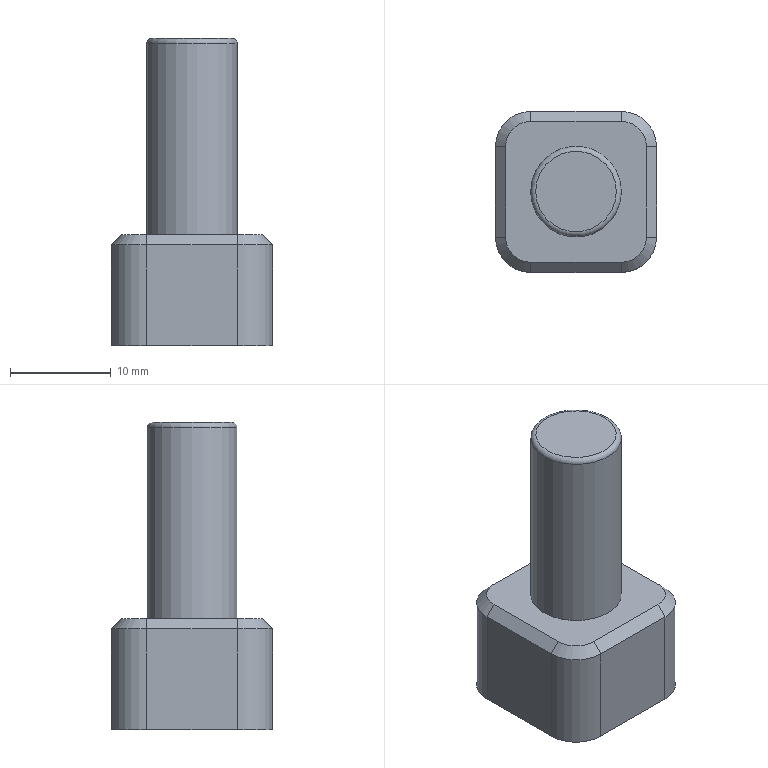Part | NX | 1 solid | 23 faces | box 16 x 16 x 30.5 mm | volume 3601 mm3 | plane 11 | cylinder 6 | cone 5 | torus 1 | commonest cylinder face diameters 7 x4 6.1 x1 9 x1
STEP:
#1=CARTESIAN_POINT('',(4.,0.,0.));
#2=VERTEX_POINT('',#1);
#3=CARTESIAN_POINT('',(0.,0.,0.));
#4=DIRECTION('',(0.,0.,1.));
#5=DIRECTION('',(1.,0.,0.));
#6=AXIS2_PLACEMENT_3D('',#3,#4,#5);
#7=CIRCLE('',#6,4.);
#8=EDGE_CURVE('',#2,#2,#7,.T.);
#9=ORIENTED_EDGE('',*,*,#8,.T.);
#10=EDGE_LOOP('',(#9));
#11=FACE_BOUND('',#10,.T.);
#12=CARTESIAN_POINT('',(0.,0.,0.));
#13=DIRECTION('',(0.,0.,1.));
#14=DIRECTION('',(1.,0.,0.));
#15=AXIS2_PLACEMENT_3D('',#12,#13,#14);
#16=PLANE('',#15);
#17=ADVANCED_FACE('',(#11),#16,.T.);
#18=CARTESIAN_POINT('',(0.,0.,-18.667));
#19=VERTEX_POINT('',#18);
#20=VERTEX_LOOP('',#19);
#21=FACE_BOUND('',#20,.T.);
#22=CARTESIAN_POINT('',(3.05,0.,-20.5));
#23=VERTEX_POINT('',#22);
#24=CARTESIAN_POINT('',(0.,0.,-20.5));
#25=DIRECTION('',(0.,0.,1.));
#26=DIRECTION('',(1.,0.,0.));
#27=AXIS2_PLACEMENT_3D('',#24,#25,#26);
#28=CIRCLE('',#27,3.05);
#29=EDGE_CURVE('',#23,#23,#28,.T.);
#30=ORIENTED_EDGE('',*,*,#29,.F.);
#31=EDGE_LOOP('',(#30));
#32=FACE_BOUND('',#31,.T.);
#33=CARTESIAN_POINT('',(0.,0.,-19.667));
#34=DIRECTION('',(0.,0.,-1.));
#35=DIRECTION('',(-1.,0.,0.));
#36=AXIS2_PLACEMENT_3D('',#33,#34,#35);
#37=CONICAL_SURFACE('',#36,1.664,1.03);
#38=ADVANCED_FACE('',(#21,#32),#37,.F.);
#39=CARTESIAN_POINT('',(3.05,0.,-30.5));
#40=VERTEX_POINT('',#39);
#41=CARTESIAN_POINT('',(0.,0.,-30.5));
#42=DIRECTION('',(0.,0.,1.));
#43=DIRECTION('',(1.,0.,0.));
#44=AXIS2_PLACEMENT_3D('',#41,#42,#43);
#45=CIRCLE('',#44,3.05);
#46=EDGE_CURVE('',#40,#40,#45,.T.);
#47=ORIENTED_EDGE('',*,*,#46,.F.);
#48=EDGE_LOOP('',(#47));
#49=FACE_BOUND('',#48,.T.);
#50=ORIENTED_EDGE('',*,*,#29,.T.);
#51=EDGE_LOOP('',(#50));
#52=FACE_BOUND('',#51,.T.);
#53=CARTESIAN_POINT('',(0.,0.,-30.5));
#54=DIRECTION('',(0.,0.,1.));
#55=DIRECTION('',(1.,0.,0.));
#56=AXIS2_PLACEMENT_3D('',#53,#54,#55);
#57=CYLINDRICAL_SURFACE('',#56,3.05);
#58=ADVANCED_FACE('',(#49,#52),#57,.F.);
#59=CARTESIAN_POINT('',(-8.,-4.5,-20.5));
#60=VERTEX_POINT('',#59);
#61=CARTESIAN_POINT('',(-7.,-4.5,-19.5));
#62=VERTEX_POINT('',#61);
#63=CARTESIAN_POINT('',(-8.,-4.5,-20.5));
#64=DIRECTION('',(0.7071,0.,0.7071));
#65=VECTOR('',#64,1000.);
#66=LINE('',#63,#65);
#67=EDGE_CURVE('',#60,#62,#66,.T.);
#68=ORIENTED_EDGE('',*,*,#67,.T.);
#69=CARTESIAN_POINT('',(-7.,4.5,-19.5));
#70=VERTEX_POINT('',#69);
#71=CARTESIAN_POINT('',(-7.,-4.5,-19.5));
#72=DIRECTION('',(0.,-1.,0.));
#73=VECTOR('',#72,1000.);
#74=LINE('',#71,#73);
#75=EDGE_CURVE('',#70,#62,#74,.T.);
#76=ORIENTED_EDGE('',*,*,#75,.F.);
#77=CARTESIAN_POINT('',(-8.,4.5,-20.5));
#78=VERTEX_POINT('',#77);
#79=CARTESIAN_POINT('',(-7.,4.5,-19.5));
#80=DIRECTION('',(-0.7071,0.,-0.7071));
#81=VECTOR('',#80,1000.);
#82=LINE('',#79,#81);
#83=EDGE_CURVE('',#70,#78,#82,.T.);
#84=ORIENTED_EDGE('',*,*,#83,.T.);
#85=CARTESIAN_POINT('',(-8.,4.5,-20.5));
#86=DIRECTION('',(0.,1.,0.));
#87=VECTOR('',#86,1000.);
#88=LINE('',#85,#87);
#89=EDGE_CURVE('',#60,#78,#88,.T.);
#90=ORIENTED_EDGE('',*,*,#89,.F.);
#91=EDGE_LOOP('',(#68,#76,#84,#90));
#92=FACE_BOUND('',#91,.T.);
#93=CARTESIAN_POINT('',(-8.,-4.5,-20.5));
#94=DIRECTION('',(-0.7071,0.,0.7071));
#95=DIRECTION('',(0.,-1.,0.));
#96=AXIS2_PLACEMENT_3D('',#93,#94,#95);
#97=PLANE('',#96);
#98=ADVANCED_FACE('',(#92),#97,.T.);
#99=CARTESIAN_POINT('',(-4.5,7.,-19.5));
#100=VERTEX_POINT('',#99);
#101=CARTESIAN_POINT('',(-4.5,8.,-20.5));
#102=VERTEX_POINT('',#101);
#103=CARTESIAN_POINT('',(-4.5,7.,-19.5));
#104=DIRECTION('',(0.,0.7071,-0.7071));
#105=VECTOR('',#104,1000.);
#106=LINE('',#103,#105);
#107=EDGE_CURVE('',#100,#102,#106,.T.);
#108=ORIENTED_EDGE('',*,*,#107,.T.);
#109=CARTESIAN_POINT('',(-4.5,4.5,-20.5));
#110=DIRECTION('',(0.,0.,1.));
#111=DIRECTION('',(1.,0.,0.));
#112=AXIS2_PLACEMENT_3D('',#109,#110,#111);
#113=CIRCLE('',#112,3.5);
#114=EDGE_CURVE('',#102,#78,#113,.T.);
#115=ORIENTED_EDGE('',*,*,#114,.T.);
#116=ORIENTED_EDGE('',*,*,#83,.F.);
#117=CARTESIAN_POINT('',(-4.5,4.5,-19.5));
#118=DIRECTION('',(0.,0.,1.));
#119=DIRECTION('',(1.,0.,0.));
#120=AXIS2_PLACEMENT_3D('',#117,#118,#119);
#121=CIRCLE('',#120,2.5);
#122=EDGE_CURVE('',#100,#70,#121,.T.);
#123=ORIENTED_EDGE('',*,*,#122,.F.);
#124=EDGE_LOOP('',(#108,#115,#116,#123));
#125=FACE_BOUND('',#124,.T.);
#126=CARTESIAN_POINT('',(-4.5,4.5,-19.5));
#127=DIRECTION('',(0.,0.,-1.));
#128=DIRECTION('',(-1.,0.,0.));
#129=AXIS2_PLACEMENT_3D('',#126,#127,#128);
#130=CONICAL_SURFACE('',#129,2.5,0.7854);
#131=ADVANCED_FACE('',(#125),#130,.T.);
#132=CARTESIAN_POINT('',(-4.5,-8.,-20.5));
#133=VERTEX_POINT('',#132);
#134=CARTESIAN_POINT('',(-4.5,-7.,-19.5));
#135=VERTEX_POINT('',#134);
#136=CARTESIAN_POINT('',(-4.5,-8.,-20.5));
#137=DIRECTION('',(0.,0.7071,0.7071));
#138=VECTOR('',#137,1000.);
#139=LINE('',#136,#138);
#140=EDGE_CURVE('',#133,#135,#139,.T.);
#141=ORIENTED_EDGE('',*,*,#140,.T.);
#142=CARTESIAN_POINT('',(-4.5,-4.5,-19.5));
#143=DIRECTION('',(0.,0.,1.));
#144=DIRECTION('',(1.,0.,0.));
#145=AXIS2_PLACEMENT_3D('',#142,#143,#144);
#146=CIRCLE('',#145,2.5);
#147=EDGE_CURVE('',#62,#135,#146,.T.);
#148=ORIENTED_EDGE('',*,*,#147,.F.);
#149=ORIENTED_EDGE('',*,*,#67,.F.);
#150=CARTESIAN_POINT('',(-4.5,-4.5,-20.5));
#151=DIRECTION('',(0.,0.,1.));
#152=DIRECTION('',(1.,0.,0.));
#153=AXIS2_PLACEMENT_3D('',#150,#151,#152);
#154=CIRCLE('',#153,3.5);
#155=EDGE_CURVE('',#60,#133,#154,.T.);
#156=ORIENTED_EDGE('',*,*,#155,.T.);
#157=EDGE_LOOP('',(#141,#148,#149,#156));
#158=FACE_BOUND('',#157,.T.);
#159=CARTESIAN_POINT('',(-4.5,-4.5,-19.5));
#160=DIRECTION('',(0.,0.,-1.));
#161=DIRECTION('',(-1.,0.,0.));
#162=AXIS2_PLACEMENT_3D('',#159,#160,#161);
#163=CONICAL_SURFACE('',#162,2.5,0.7854);
#164=ADVANCED_FACE('',(#158),#163,.T.);
#165=CARTESIAN_POINT('',(4.5,7.,-19.5));
#166=VERTEX_POINT('',#165);
#167=CARTESIAN_POINT('',(4.5,8.,-20.5));
#168=VERTEX_POINT('',#167);
#169=CARTESIAN_POINT('',(4.5,7.,-19.5));
#170=DIRECTION('',(0.,0.7071,-0.7071));
#171=VECTOR('',#170,1000.);
#172=LINE('',#169,#171);
#173=EDGE_CURVE('',#166,#168,#172,.T.);
#174=ORIENTED_EDGE('',*,*,#173,.T.);
#175=CARTESIAN_POINT('',(4.5,8.,-20.5));
#176=DIRECTION('',(1.,0.,0.));
#177=VECTOR('',#176,1000.);
#178=LINE('',#175,#177);
#179=EDGE_CURVE('',#102,#168,#178,.T.);
#180=ORIENTED_EDGE('',*,*,#179,.F.);
#181=ORIENTED_EDGE('',*,*,#107,.F.);
#182=CARTESIAN_POINT('',(-4.5,7.,-19.5));
#183=DIRECTION('',(-1.,0.,0.));
#184=VECTOR('',#183,1000.);
#185=LINE('',#182,#184);
#186=EDGE_CURVE('',#166,#100,#185,.T.);
#187=ORIENTED_EDGE('',*,*,#186,.F.);
#188=EDGE_LOOP('',(#174,#180,#181,#187));
#189=FACE_BOUND('',#188,.T.);
#190=CARTESIAN_POINT('',(-4.5,8.,-20.5));
#191=DIRECTION('',(0.,0.7071,0.7071));
#192=DIRECTION('',(-1.,0.,0.));
#193=AXIS2_PLACEMENT_3D('',#190,#191,#192);
#194=PLANE('',#193);
#195=ADVANCED_FACE('',(#189),#194,.T.);
#196=CARTESIAN_POINT('',(4.5,-8.,-20.5));
#197=VERTEX_POINT('',#196);
#198=CARTESIAN_POINT('',(4.5,-7.,-19.5));
#199=VERTEX_POINT('',#198);
#200=CARTESIAN_POINT('',(4.5,-8.,-20.5));
#201=DIRECTION('',(0.,0.7071,0.7071));
#202=VECTOR('',#201,1000.);
#203=LINE('',#200,#202);
#204=EDGE_CURVE('',#197,#199,#203,.T.);
#205=ORIENTED_EDGE('',*,*,#204,.T.);
#206=CARTESIAN_POINT('',(4.5,-7.,-19.5));
#207=DIRECTION('',(1.,0.,0.));
#208=VECTOR('',#207,1000.);
#209=LINE('',#206,#208);
#210=EDGE_CURVE('',#135,#199,#209,.T.);
#211=ORIENTED_EDGE('',*,*,#210,.F.);
#212=ORIENTED_EDGE('',*,*,#140,.F.);
#213=CARTESIAN_POINT('',(-4.5,-8.,-20.5));
#214=DIRECTION('',(-1.,0.,0.));
#215=VECTOR('',#214,1000.);
#216=LINE('',#213,#215);
#217=EDGE_CURVE('',#197,#133,#216,.T.);
#218=ORIENTED_EDGE('',*,*,#217,.F.);
#219=EDGE_LOOP('',(#205,#211,#212,#218));
#220=FACE_BOUND('',#219,.T.);
#221=CARTESIAN_POINT('',(4.5,-8.,-20.5));
#222=DIRECTION('',(0.,-0.7071,0.7071));
#223=DIRECTION('',(1.,0.,0.));
#224=AXIS2_PLACEMENT_3D('',#221,#222,#223);
#225=PLANE('',#224);
#226=ADVANCED_FACE('',(#220),#225,.T.);
#227=CARTESIAN_POINT('',(7.,4.5,-19.5));
#228=VERTEX_POINT('',#227);
#229=CARTESIAN_POINT('',(8.,4.5,-20.5));
#230=VERTEX_POINT('',#229);
#231=CARTESIAN_POINT('',(7.,4.5,-19.5));
#232=DIRECTION('',(0.7071,0.,-0.7071));
#233=VECTOR('',#232,1000.);
#234=LINE('',#231,#233);
#235=EDGE_CURVE('',#228,#230,#234,.T.);
#236=ORIENTED_EDGE('',*,*,#235,.T.);
#237=CARTESIAN_POINT('',(4.5,4.5,-20.5));
#238=DIRECTION('',(0.,0.,1.));
#239=DIRECTION('',(1.,0.,0.));
#240=AXIS2_PLACEMENT_3D('',#237,#238,#239);
#241=CIRCLE('',#240,3.5);
#242=EDGE_CURVE('',#230,#168,#241,.T.);
#243=ORIENTED_EDGE('',*,*,#242,.T.);
#244=ORIENTED_EDGE('',*,*,#173,.F.);
#245=CARTESIAN_POINT('',(4.5,4.5,-19.5));
#246=DIRECTION('',(0.,0.,1.));
#247=DIRECTION('',(1.,0.,0.));
#248=AXIS2_PLACEMENT_3D('',#245,#246,#247);
#249=CIRCLE('',#248,2.5);
#250=EDGE_CURVE('',#228,#166,#249,.T.);
#251=ORIENTED_EDGE('',*,*,#250,.F.);
#252=EDGE_LOOP('',(#236,#243,#244,#251));
#253=FACE_BOUND('',#252,.T.);
#254=CARTESIAN_POINT('',(4.5,4.5,-19.5));
#255=DIRECTION('',(0.,0.,-1.));
#256=DIRECTION('',(-1.,0.,0.));
#257=AXIS2_PLACEMENT_3D('',#254,#255,#256);
#258=CONICAL_SURFACE('',#257,2.5,0.7854);
#259=ADVANCED_FACE('',(#253),#258,.T.);
#260=CARTESIAN_POINT('',(8.,-4.5,-20.5));
#261=VERTEX_POINT('',#260);
#262=CARTESIAN_POINT('',(7.,-4.5,-19.5));
#263=VERTEX_POINT('',#262);
#264=CARTESIAN_POINT('',(8.,-4.5,-20.5));
#265=DIRECTION('',(-0.7071,0.,0.7071));
#266=VECTOR('',#265,1000.);
#267=LINE('',#264,#266);
#268=EDGE_CURVE('',#261,#263,#267,.T.);
#269=ORIENTED_EDGE('',*,*,#268,.T.);
#270=CARTESIAN_POINT('',(4.5,-4.5,-19.5));
#271=DIRECTION('',(0.,0.,1.));
#272=DIRECTION('',(1.,0.,0.));
#273=AXIS2_PLACEMENT_3D('',#270,#271,#272);
#274=CIRCLE('',#273,2.5);
#275=EDGE_CURVE('',#199,#263,#274,.T.);
#276=ORIENTED_EDGE('',*,*,#275,.F.);
#277=ORIENTED_EDGE('',*,*,#204,.F.);
#278=CARTESIAN_POINT('',(4.5,-4.5,-20.5));
#279=DIRECTION('',(0.,0.,1.));
#280=DIRECTION('',(1.,0.,0.));
#281=AXIS2_PLACEMENT_3D('',#278,#279,#280);
#282=CIRCLE('',#281,3.5);
#283=EDGE_CURVE('',#197,#261,#282,.T.);
#284=ORIENTED_EDGE('',*,*,#283,.T.);
#285=EDGE_LOOP('',(#269,#276,#277,#284));
#286=FACE_BOUND('',#285,.T.);
#287=CARTESIAN_POINT('',(4.5,-4.5,-19.5));
#288=DIRECTION('',(0.,0.,-1.));
#289=DIRECTION('',(-1.,0.,0.));
#290=AXIS2_PLACEMENT_3D('',#287,#288,#289);
#291=CONICAL_SURFACE('',#290,2.5,0.7854);
#292=ADVANCED_FACE('',(#286),#291,.T.);
#293=ORIENTED_EDGE('',*,*,#235,.F.);
#294=CARTESIAN_POINT('',(7.,4.5,-19.5));
#295=DIRECTION('',(0.,1.,0.));
#296=VECTOR('',#295,1000.);
#297=LINE('',#294,#296);
#298=EDGE_CURVE('',#263,#228,#297,.T.);
#299=ORIENTED_EDGE('',*,*,#298,.F.);
#300=ORIENTED_EDGE('',*,*,#268,.F.);
#301=CARTESIAN_POINT('',(8.,-4.5,-20.5));
#302=DIRECTION('',(0.,-1.,0.));
#303=VECTOR('',#302,1000.);
#304=LINE('',#301,#303);
#305=EDGE_CURVE('',#230,#261,#304,.T.);
#306=ORIENTED_EDGE('',*,*,#305,.F.);
#307=EDGE_LOOP('',(#293,#299,#300,#306));
#308=FACE_BOUND('',#307,.T.);
#309=CARTESIAN_POINT('',(8.,4.5,-20.5));
#310=DIRECTION('',(0.7071,0.,0.7071));
#311=DIRECTION('',(0.,1.,0.));
#312=AXIS2_PLACEMENT_3D('',#309,#310,#311);
#313=PLANE('',#312);
#314=ADVANCED_FACE('',(#308),#313,.T.);
#315=CARTESIAN_POINT('',(4.5,0.,-0.5));
#316=VERTEX_POINT('',#315);
#317=CARTESIAN_POINT('',(0.,0.,-0.5));
#318=DIRECTION('',(0.,0.,1.));
#319=DIRECTION('',(1.,0.,0.));
#320=AXIS2_PLACEMENT_3D('',#317,#318,#319);
#321=CIRCLE('',#320,4.5);
#322=EDGE_CURVE('',#316,#316,#321,.F.);
#323=ORIENTED_EDGE('',*,*,#322,.T.);
#324=EDGE_LOOP('',(#323));
#325=FACE_BOUND('',#324,.T.);
#326=CARTESIAN_POINT('',(4.5,0.,-19.5));
#327=VERTEX_POINT('',#326);
#328=CARTESIAN_POINT('',(0.,0.,-19.5));
#329=DIRECTION('',(0.,0.,1.));
#330=DIRECTION('',(1.,0.,0.));
#331=AXIS2_PLACEMENT_3D('',#328,#329,#330);
#332=CIRCLE('',#331,4.5);
#333=EDGE_CURVE('',#327,#327,#332,.T.);
#334=ORIENTED_EDGE('',*,*,#333,.T.);
#335=EDGE_LOOP('',(#334));
#336=FACE_BOUND('',#335,.T.);
#337=CARTESIAN_POINT('',(0.,0.,0.));
#338=DIRECTION('',(0.,0.,-1.));
#339=DIRECTION('',(-1.,0.,0.));
#340=AXIS2_PLACEMENT_3D('',#337,#338,#339);
#341=CYLINDRICAL_SURFACE('',#340,4.5);
#342=ADVANCED_FACE('',(#325,#336),#341,.T.);
#343=ORIENTED_EDGE('',*,*,#333,.F.);
#344=EDGE_LOOP('',(#343));
#345=FACE_BOUND('',#344,.T.);
#346=ORIENTED_EDGE('',*,*,#122,.T.);
#347=ORIENTED_EDGE('',*,*,#75,.T.);
#348=ORIENTED_EDGE('',*,*,#147,.T.);
#349=ORIENTED_EDGE('',*,*,#210,.T.);
#350=ORIENTED_EDGE('',*,*,#275,.T.);
#351=ORIENTED_EDGE('',*,*,#298,.T.);
#352=ORIENTED_EDGE('',*,*,#250,.T.);
#353=ORIENTED_EDGE('',*,*,#186,.T.);
#354=EDGE_LOOP('',(#346,#347,#348,#349,#350,#351,#352,#353));
#355=FACE_BOUND('',#354,.T.);
#356=CARTESIAN_POINT('',(4.5,-4.5,-19.5));
#357=DIRECTION('',(0.,0.,1.));
#358=DIRECTION('',(1.,0.,0.));
#359=AXIS2_PLACEMENT_3D('',#356,#357,#358);
#360=PLANE('',#359);
#361=ADVANCED_FACE('',(#345,#355),#360,.T.);
#362=ORIENTED_EDGE('',*,*,#46,.T.);
#363=EDGE_LOOP('',(#362));
#364=FACE_BOUND('',#363,.T.);
#365=CARTESIAN_POINT('',(4.5,-8.,-30.5));
#366=VERTEX_POINT('',#365);
#367=CARTESIAN_POINT('',(8.,-4.5,-30.5));
#368=VERTEX_POINT('',#367);
#369=CARTESIAN_POINT('',(4.5,-4.5,-30.5));
#370=DIRECTION('',(0.,0.,1.));
#371=DIRECTION('',(1.,0.,0.));
#372=AXIS2_PLACEMENT_3D('',#369,#370,#371);
#373=CIRCLE('',#372,3.5);
#374=EDGE_CURVE('',#366,#368,#373,.T.);
#375=ORIENTED_EDGE('',*,*,#374,.F.);
#376=CARTESIAN_POINT('',(-4.5,-8.,-30.5));
#377=VERTEX_POINT('',#376);
#378=CARTESIAN_POINT('',(4.5,-8.,-30.5));
#379=DIRECTION('',(-1.,0.,0.));
#380=VECTOR('',#379,1000.);
#381=LINE('',#378,#380);
#382=EDGE_CURVE('',#366,#377,#381,.T.);
#383=ORIENTED_EDGE('',*,*,#382,.T.);
#384=CARTESIAN_POINT('',(-8.,-4.5,-30.5));
#385=VERTEX_POINT('',#384);
#386=CARTESIAN_POINT('',(-4.5,-4.5,-30.5));
#387=DIRECTION('',(0.,0.,1.));
#388=DIRECTION('',(1.,0.,0.));
#389=AXIS2_PLACEMENT_3D('',#386,#387,#388);
#390=CIRCLE('',#389,3.5);
#391=EDGE_CURVE('',#385,#377,#390,.T.);
#392=ORIENTED_EDGE('',*,*,#391,.F.);
#393=CARTESIAN_POINT('',(-8.,4.5,-30.5));
#394=VERTEX_POINT('',#393);
#395=CARTESIAN_POINT('',(-8.,-4.5,-30.5));
#396=DIRECTION('',(0.,1.,0.));
#397=VECTOR('',#396,1000.);
#398=LINE('',#395,#397);
#399=EDGE_CURVE('',#385,#394,#398,.T.);
#400=ORIENTED_EDGE('',*,*,#399,.T.);
#401=CARTESIAN_POINT('',(-4.5,8.,-30.5));
#402=VERTEX_POINT('',#401);
#403=CARTESIAN_POINT('',(-4.5,4.5,-30.5));
#404=DIRECTION('',(0.,0.,1.));
#405=DIRECTION('',(1.,0.,0.));
#406=AXIS2_PLACEMENT_3D('',#403,#404,#405);
#407=CIRCLE('',#406,3.5);
#408=EDGE_CURVE('',#402,#394,#407,.T.);
#409=ORIENTED_EDGE('',*,*,#408,.F.);
#410=CARTESIAN_POINT('',(4.5,8.,-30.5));
#411=VERTEX_POINT('',#410);
#412=CARTESIAN_POINT('',(-4.5,8.,-30.5));
#413=DIRECTION('',(1.,0.,0.));
#414=VECTOR('',#413,1000.);
#415=LINE('',#412,#414);
#416=EDGE_CURVE('',#402,#411,#415,.T.);
#417=ORIENTED_EDGE('',*,*,#416,.T.);
#418=CARTESIAN_POINT('',(8.,4.5,-30.5));
#419=VERTEX_POINT('',#418);
#420=CARTESIAN_POINT('',(4.5,4.5,-30.5));
#421=DIRECTION('',(0.,0.,1.));
#422=DIRECTION('',(1.,0.,0.));
#423=AXIS2_PLACEMENT_3D('',#420,#421,#422);
#424=CIRCLE('',#423,3.5);
#425=EDGE_CURVE('',#419,#411,#424,.T.);
#426=ORIENTED_EDGE('',*,*,#425,.F.);
#427=CARTESIAN_POINT('',(8.,4.5,-30.5));
#428=DIRECTION('',(0.,-1.,0.));
#429=VECTOR('',#428,1000.);
#430=LINE('',#427,#429);
#431=EDGE_CURVE('',#419,#368,#430,.T.);
#432=ORIENTED_EDGE('',*,*,#431,.T.);
#433=EDGE_LOOP('',(#375,#383,#392,#400,#409,#417,#426,#432));
#434=FACE_BOUND('',#433,.T.);
#435=CARTESIAN_POINT('',(4.5,-4.5,-30.5));
#436=DIRECTION('',(0.,0.,1.));
#437=DIRECTION('',(1.,0.,0.));
#438=AXIS2_PLACEMENT_3D('',#435,#436,#437);
#439=PLANE('',#438);
#440=ADVANCED_FACE('',(#364,#434),#439,.F.);
#441=CARTESIAN_POINT('',(4.5,-8.,-30.5));
#442=DIRECTION('',(0.,0.,1.));
#443=VECTOR('',#442,1000.);
#444=LINE('',#441,#443);
#445=EDGE_CURVE('',#366,#197,#444,.T.);
#446=ORIENTED_EDGE('',*,*,#445,.T.);
#447=ORIENTED_EDGE('',*,*,#217,.T.);
#448=CARTESIAN_POINT('',(-4.5,-8.,-30.5));
#449=DIRECTION('',(0.,0.,1.));
#450=VECTOR('',#449,1000.);
#451=LINE('',#448,#450);
#452=EDGE_CURVE('',#377,#133,#451,.T.);
#453=ORIENTED_EDGE('',*,*,#452,.F.);
#454=ORIENTED_EDGE('',*,*,#382,.F.);
#455=EDGE_LOOP('',(#446,#447,#453,#454));
#456=FACE_BOUND('',#455,.T.);
#457=CARTESIAN_POINT('',(4.5,-8.,-30.5));
#458=DIRECTION('',(0.,1.,0.));
#459=DIRECTION('',(-1.,0.,0.));
#460=AXIS2_PLACEMENT_3D('',#457,#458,#459);
#461=PLANE('',#460);
#462=ADVANCED_FACE('',(#456),#461,.F.);
#463=ORIENTED_EDGE('',*,*,#452,.T.);
#464=ORIENTED_EDGE('',*,*,#155,.F.);
#465=CARTESIAN_POINT('',(-8.,-4.5,-30.5));
#466=DIRECTION('',(0.,0.,1.));
#467=VECTOR('',#466,1000.);
#468=LINE('',#465,#467);
#469=EDGE_CURVE('',#385,#60,#468,.T.);
#470=ORIENTED_EDGE('',*,*,#469,.F.);
#471=ORIENTED_EDGE('',*,*,#391,.T.);
#472=EDGE_LOOP('',(#463,#464,#470,#471));
#473=FACE_BOUND('',#472,.T.);
#474=CARTESIAN_POINT('',(-4.5,-4.5,-30.5));
#475=DIRECTION('',(0.,0.,1.));
#476=DIRECTION('',(1.,0.,0.));
#477=AXIS2_PLACEMENT_3D('',#474,#475,#476);
#478=CYLINDRICAL_SURFACE('',#477,3.5);
#479=ADVANCED_FACE('',(#473),#478,.T.);
#480=ORIENTED_EDGE('',*,*,#469,.T.);
#481=ORIENTED_EDGE('',*,*,#89,.T.);
#482=CARTESIAN_POINT('',(-8.,4.5,-30.5));
#483=DIRECTION('',(0.,0.,1.));
#484=VECTOR('',#483,1000.);
#485=LINE('',#482,#484);
#486=EDGE_CURVE('',#394,#78,#485,.T.);
#487=ORIENTED_EDGE('',*,*,#486,.F.);
#488=ORIENTED_EDGE('',*,*,#399,.F.);
#489=EDGE_LOOP('',(#480,#481,#487,#488));
#490=FACE_BOUND('',#489,.T.);
#491=CARTESIAN_POINT('',(-8.,-4.5,-30.5));
#492=DIRECTION('',(1.,0.,0.));
#493=DIRECTION('',(0.,0.,-1.));
#494=AXIS2_PLACEMENT_3D('',#491,#492,#493);
#495=PLANE('',#494);
#496=ADVANCED_FACE('',(#490),#495,.F.);
#497=ORIENTED_EDGE('',*,*,#486,.T.);
#498=ORIENTED_EDGE('',*,*,#114,.F.);
#499=CARTESIAN_POINT('',(-4.5,8.,-30.5));
#500=DIRECTION('',(0.,0.,1.));
#501=VECTOR('',#500,1000.);
#502=LINE('',#499,#501);
#503=EDGE_CURVE('',#402,#102,#502,.T.);
#504=ORIENTED_EDGE('',*,*,#503,.F.);
#505=ORIENTED_EDGE('',*,*,#408,.T.);
#506=EDGE_LOOP('',(#497,#498,#504,#505));
#507=FACE_BOUND('',#506,.T.);
#508=CARTESIAN_POINT('',(-4.5,4.5,-30.5));
#509=DIRECTION('',(0.,0.,1.));
#510=DIRECTION('',(1.,0.,0.));
#511=AXIS2_PLACEMENT_3D('',#508,#509,#510);
#512=CYLINDRICAL_SURFACE('',#511,3.5);
#513=ADVANCED_FACE('',(#507),#512,.T.);
#514=ORIENTED_EDGE('',*,*,#503,.T.);
#515=ORIENTED_EDGE('',*,*,#179,.T.);
#516=CARTESIAN_POINT('',(4.5,8.,-30.5));
#517=DIRECTION('',(0.,0.,1.));
#518=VECTOR('',#517,1000.);
#519=LINE('',#516,#518);
#520=EDGE_CURVE('',#411,#168,#519,.T.);
#521=ORIENTED_EDGE('',*,*,#520,.F.);
#522=ORIENTED_EDGE('',*,*,#416,.F.);
#523=EDGE_LOOP('',(#514,#515,#521,#522));
#524=FACE_BOUND('',#523,.T.);
#525=CARTESIAN_POINT('',(-4.5,8.,-30.5));
#526=DIRECTION('',(0.,-1.,0.));
#527=DIRECTION('',(1.,0.,0.));
#528=AXIS2_PLACEMENT_3D('',#525,#526,#527);
#529=PLANE('',#528);
#530=ADVANCED_FACE('',(#524),#529,.F.);
#531=ORIENTED_EDGE('',*,*,#520,.T.);
#532=ORIENTED_EDGE('',*,*,#242,.F.);
#533=CARTESIAN_POINT('',(8.,4.5,-30.5));
#534=DIRECTION('',(0.,0.,1.));
#535=VECTOR('',#534,1000.);
#536=LINE('',#533,#535);
#537=EDGE_CURVE('',#419,#230,#536,.T.);
#538=ORIENTED_EDGE('',*,*,#537,.F.);
#539=ORIENTED_EDGE('',*,*,#425,.T.);
#540=EDGE_LOOP('',(#531,#532,#538,#539));
#541=FACE_BOUND('',#540,.T.);
#542=CARTESIAN_POINT('',(4.5,4.5,-30.5));
#543=DIRECTION('',(0.,0.,1.));
#544=DIRECTION('',(1.,0.,0.));
#545=AXIS2_PLACEMENT_3D('',#542,#543,#544);
#546=CYLINDRICAL_SURFACE('',#545,3.5);
#547=ADVANCED_FACE('',(#541),#546,.T.);
#548=ORIENTED_EDGE('',*,*,#537,.T.);
#549=ORIENTED_EDGE('',*,*,#305,.T.);
#550=CARTESIAN_POINT('',(8.,-4.5,-30.5));
#551=DIRECTION('',(0.,0.,1.));
#552=VECTOR('',#551,1000.);
#553=LINE('',#550,#552);
#554=EDGE_CURVE('',#368,#261,#553,.T.);
#555=ORIENTED_EDGE('',*,*,#554,.F.);
#556=ORIENTED_EDGE('',*,*,#431,.F.);
#557=EDGE_LOOP('',(#548,#549,#555,#556));
#558=FACE_BOUND('',#557,.T.);
#559=CARTESIAN_POINT('',(8.,4.5,-30.5));
#560=DIRECTION('',(-1.,0.,0.));
#561=DIRECTION('',(0.,-1.,0.));
#562=AXIS2_PLACEMENT_3D('',#559,#560,#561);
#563=PLANE('',#562);
#564=ADVANCED_FACE('',(#558),#563,.F.);
#565=ORIENTED_EDGE('',*,*,#554,.T.);
#566=ORIENTED_EDGE('',*,*,#283,.F.);
#567=ORIENTED_EDGE('',*,*,#445,.F.);
#568=ORIENTED_EDGE('',*,*,#374,.T.);
#569=EDGE_LOOP('',(#565,#566,#567,#568));
#570=FACE_BOUND('',#569,.T.);
#571=CARTESIAN_POINT('',(4.5,-4.5,-30.5));
#572=DIRECTION('',(0.,0.,1.));
#573=DIRECTION('',(1.,0.,0.));
#574=AXIS2_PLACEMENT_3D('',#571,#572,#573);
#575=CYLINDRICAL_SURFACE('',#574,3.5);
#576=ADVANCED_FACE('',(#570),#575,.T.);
#577=ORIENTED_EDGE('',*,*,#322,.F.);
#578=EDGE_LOOP('',(#577));
#579=FACE_BOUND('',#578,.T.);
#580=ORIENTED_EDGE('',*,*,#8,.F.);
#581=EDGE_LOOP('',(#580));
#582=FACE_BOUND('',#581,.T.);
#583=CARTESIAN_POINT('',(0.,0.,-0.5));
#584=DIRECTION('',(0.,0.,1.));
#585=DIRECTION('',(1.,0.,0.));
#586=AXIS2_PLACEMENT_3D('',#583,#584,#585);
#587=TOROIDAL_SURFACE('',#586,4.,0.5);
#588=ADVANCED_FACE('',(#579,#582),#587,.T.);
#589=CLOSED_SHELL('',(#17,#38,#58,#98,#131,#164,#195,#226,#259,#292,#314,#342,#361,#440,#462,#479,#496,#513,#530,#547,#564,#576,#588));
#590=MANIFOLD_SOLID_BREP('',#589);
#591=(LENGTH_UNIT()NAMED_UNIT(*)SI_UNIT(.MILLI.,.METRE.));
#592=UNCERTAINTY_MEASURE_WITH_UNIT(LENGTH_MEASURE(0.00001),#591,'','');
#593=(NAMED_UNIT(*)PLANE_ANGLE_UNIT()SI_UNIT($,.RADIAN.));
#594=(NAMED_UNIT(*)SI_UNIT($,.STERADIAN.)SOLID_ANGLE_UNIT());
#595=(GEOMETRIC_REPRESENTATION_CONTEXT(3)GLOBAL_UNCERTAINTY_ASSIGNED_CONTEXT((#592))GLOBAL_UNIT_ASSIGNED_CONTEXT((#591,#593,#594))REPRESENTATION_CONTEXT('',''));
#596=ADVANCED_BREP_SHAPE_REPRESENTATION('',(#590),#595);